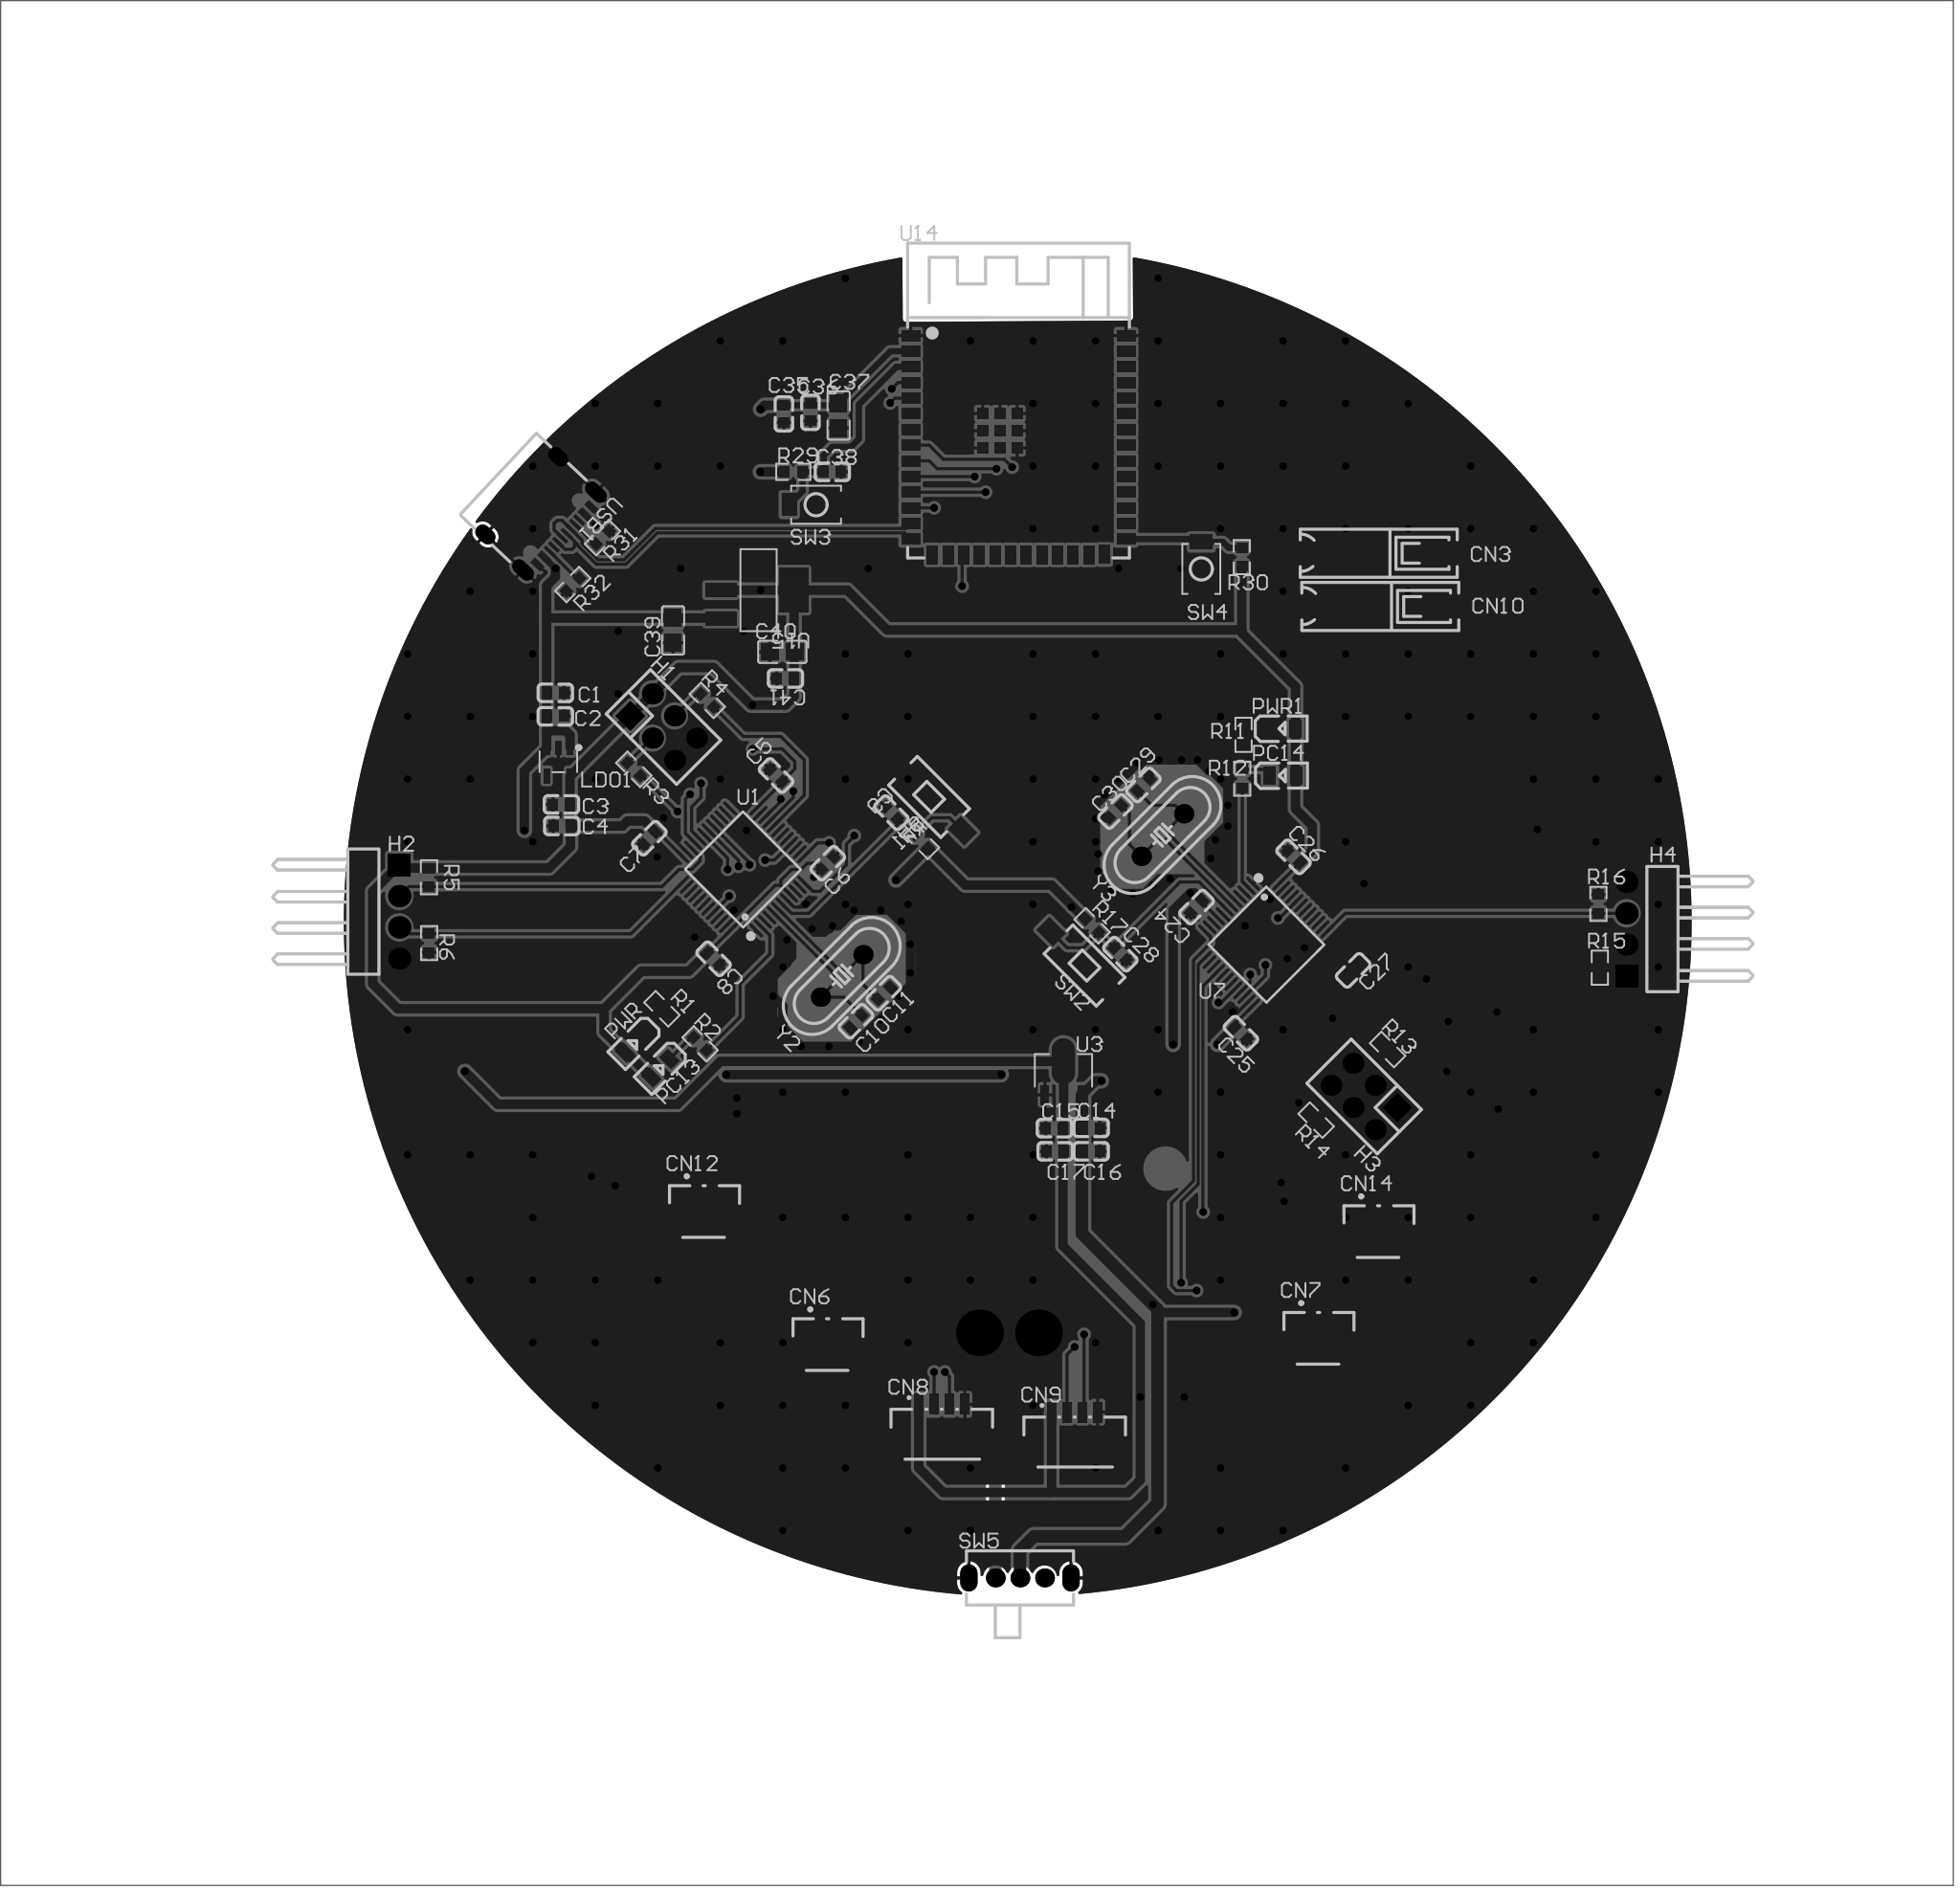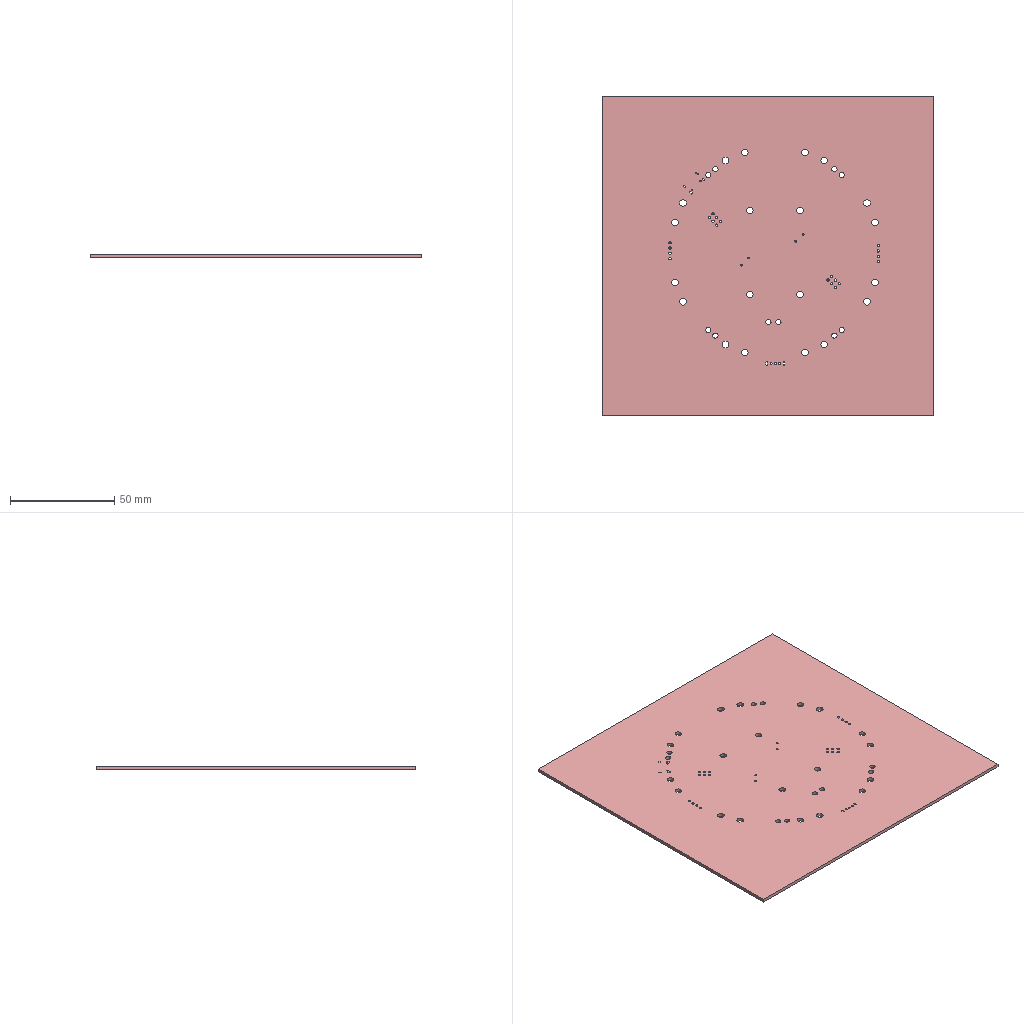Circuit board layout | Altium Designer | box 158.6 x 152.9 x 1.6 mm
Layer stack:
# Altium Designer layer stack of  (unit mm; dielectric type: 0 none, 1 core, 2 prepreg, 3 surface material)
index,name,kind,layer,copper_thickness_mm,dielectric_type,dielectric_thickness_mm,dielectric_material,dielectric_constant
0,Top Paste Mask Layer,other,,,,,,
1,Top Silkscreen Layer,other,,,,,,
2,Top Solder Mask Layer,dielectric,,,3,0.01,,3.3
3,Top Layer,copper,Top Layer,0.035,,,,
4,Dielectric1,dielectric,,,3,1.51,FR4,4.5
5,Bottom Layer,copper,Bottom Layer,0.035,,,,
6,Bottom Solder Mask Layer,dielectric,,,3,0.01,,3.3
7,Bottom Silkscreen Layer,other,,,,,,
8,Bottom Paste Mask Layer,other,,,,,,
# drill layer pairs: low layer,high layer
drill_pair,Top Layer,Bottom Layer
Part placement:
Designator,Comment,Layer,Footprint,Center-X(mm),Center-Y(mm),Rotation
C1,CAPCER0.1UF16VX5R0603,CAPCER0.1UF25VX5R0603,CAPCER0.1UF16VX7R0603,TopLayer,C0603,114.901,166.604,180
C2,1uF,TopLayer,C0603,114.901,164.699,180
C3,1uF,TopLayer,C0603,115.411,157.549,0
C4,CAPCER0.1UF16VX5R0603,CAPCER0.1UF25VX5R0603,CAPCER0.1UF16VX7R0603,TopLayer,C0603,115.442,155.796,0
C5,100nF,TopLayer,C0603,132.842,159.893,315
C6,100nF,TopLayer,C0603,137.033,152.781,225
C7,100nF,TopLayer,C0603,122.555,154.813,45
C8,100nF,TopLayer,C0603,127.762,145.034,135
C9,CAPCER0.1UF16VX5R0603,CAPCER0.1UF25VX5R0603,CAPCER0.1UF16VX7R0603,TopLayer,C0603,142.214,156.871,315
C10,18pF,TopLayer,C0603,139.319,139.954,225
C11,18pF,TopLayer,C0603,141.605,142.24,45
C14,100nF,TopLayer,C0603,158.428,131.313,180
C15,100nF,TopLayer,C0603,155.446,131.285,180
C16,10uF,TopLayer,C0603,158.428,129.408,180
C17,22uF,TopLayer,C0603,155.507,129.408,180
C18,30pF,BottomLayer,C0805,112.402,137.656,90
C19,30pF,BottomLayer,C0805,114.561,137.656,90
C24,100nF,TopLayer,C0603,167.005,149.225,45
C25,100nF,TopLayer,C0603,170.6,138.994,135
C26,100nF,TopLayer,C0603,174.879,153.289,315
C27,100nF,TopLayer,C0603,179.718,144.083,225
C28,CAPCER0.1UF16VX5R0603,CAPCER0.1UF25VX5R0603,CAPCER0.1UF16VX7R0603,TopLayer,C0603,160.805,145.414,135
C29,18pF,TopLayer,C0603,162.687,159.131,45
C30,18pF,TopLayer,C0603,160.401,156.972,225
C33,30pF,BottomLayer,C0805,193.421,154.432,90
C34,30pF,BottomLayer,C0805,189.077,158.454,270
C35,100nF,TopLayer,C0603,133.477,189.23,90
C36,100nF,TopLayer,C0603,135.636,189.357,90
C37,10uF,TopLayer,C0805,137.922,189.103,90
C38,100nF,TopLayer,C0603,137.414,184.531,180
C39,10uF,TopLayer,C0805,124.473,171.666,90
C40,22uF,TopLayer,C0805,133.35,169.926,0
C41,100nF,TopLayer,C0603,133.604,167.767,180
CN1,WAFER-GH1.25-3PLB,BottomLayer,CONN-SMD_3P-P1.25_XUNPU_WAFER-GH1.25-3PLB,126.746,117.094,180
CN2,WAFER-GH1.25-3PLB,BottomLayer,CONN-SMD_3P-P1.25_XUNPU_WAFER-GH1.25-3PLB,163.449,122.195,180
CN3,2060-451/998-404,TopLayer,CONN-SMD_L12.7-W3.9_2060-451-998-404,182.499,177.927,0
CN4,WAFER-GH1.25-2PLB,BottomLayer,CONN-TH_2P-P1.25_XUNPU_WAFER-GH1.25-2PLB,135.763,122.047,180
CN5,WAFER-GH1.25-2PLB,BottomLayer,CONN-TH_2P-P1.25_XUNPU_WAFER-GH1.25-2PLB,166.37,114.808,180
CN6,WAFER-GH1.25-2PLB,TopLayer,CONN-TH_2P-P1.25_XUNPU_WAFER-GH1.25-2PLB,137.033,114.427,0
CN7,WAFER-GH1.25-2PLB,TopLayer,CONN-TH_2P-P1.25_XUNPU_WAFER-GH1.25-2PLB,176.911,114.935,0
CN10,2060-451/998-404,TopLayer,CONN-SMD_L12.7-W3.9_2060-451-998-404,182.626,173.609,0
CN11,GH1.25-2P,BottomLayer,CONN-TH_2P-P1.25_XUNPU_WAFER-GH1.25-2PLB,119.126,122.682,180
CN12,GH1.25-2P,TopLayer,CONN-TH_2P-P1.25_XUNPU_WAFER-GH1.25-2PLB,127,125.222,0
CN13,GH1.25-2P,BottomLayer,CONN-TH_2P-P1.25_XUNPU_WAFER-GH1.25-2PLB,173.482,121.412,180
CN14,GH1.25-2P,TopLayer,CONN-TH_2P-P1.25_XUNPU_WAFER-GH1.25-2PLB,181.787,123.592,0
H1,PZ254V-12-6P,TopLayer,HDR-TH_6P-P2.54-V-M-R2-C3-S2.54,123.698,163.83,315
H2,2541WR-04P,TopLayer,HDR-TH_4P-P2.54-H-M-W10.4-N,102.235,148.844,270
H3,PZ254V-12-6P,TopLayer,HDR-TH_6P-P2.54-V-M-R2-C3-S2.54,180.617,133.857,135
H4,2541WR-04P,TopLayer,HDR-TH_4P-P2.54-H-M-W10.4-N,201.93,147.447,90
LDO1,ME6211C33M5G-N,TopLayer,SOT-23-5_L3.0-W1.7-P0.95-LS2.8-BL,115.156,161.016,180
PC13,NCD0805R1,TopLayer,LED0805-R-RD,123.444,136.144,225
PC14,NCD0805R1,TopLayer,LED0805-R-RD,174.013,159.892,0
PWR,NCD0805R1,TopLayer,LED0805-R-RD,121.306,138.167,225
PWR1,NCD0805R1,TopLayer,LED0805-R-RD,173.99,163.703,0
Q1,STD12NF06LT4,BottomLayer,TO-252-3_L6.5-W5.8-P4.58-BL,122.816,145.785,180
Q2,STD12NF06LT4,BottomLayer,TO-252-3_L6.5-W5.8-P4.58-BL,179.959,150.241,0
Q3,STD12NF06LT4,BottomLayer,TO-252-3_L6.5-W5.8-P4.58-BL,122.963,132.762,180
Q4,STD12NF06LT4,BottomLayer,TO-252-3_L6.5-W5.8-P4.58-BL,179.912,163.349,0
R1,10kΩ,TopLayer,R0603,123.571,140.97,135
R2,10kΩ,TopLayer,R0603,126.668,138.127,315
R3,10kΩ,TopLayer,R0603,121.285,160.401,135
R4,10kΩ,TopLayer,R0603,127.254,165.989,315
R5,10kΩ,TopLayer,R0603,104.648,151.638,90
R6,10kΩ,TopLayer,R0603,104.661,146.301,90
R7,10kΩ,TopLayer,R0603,144.653,154.559,315
R8,0Ω,BottomLayer,R0805,112.402,141.72,270
R9,0Ω,BottomLayer,R0805,114.561,141.72,270
R10,120Ω,BottomLayer,R0805,116.72,139.308,90
R11,10kΩ,TopLayer,R0603,170.815,163.195,270
R12,10kΩ,TopLayer,R0603,170.711,159.638,270
R13,10kΩ,TopLayer,R0603,182.522,137.667,315
R14,10kΩ,TopLayer,R0603,176.714,131.937,135
R15,10kΩ,TopLayer,R0603,199.758,144.304,270
R16,10kΩ,TopLayer,R0603,199.644,149.479,270
R17,10kΩ,TopLayer,R0603,158.519,147.7,135
R18,0Ω,BottomLayer,R0805,191.236,154.391,90
R19,0Ω,BottomLayer,R0805,189.077,154.391,90
R20,120Ω,BottomLayer,R0805,186.944,158.369,90
R21,10kΩ,BottomLayer,R0603,116.84,142.748,90
R22,10kΩ,BottomLayer,R0603,186.77,154.332,270
R27,1kΩ,BottomLayer,R0805,128.805,141.017,270
R28,1kΩ,BottomLayer,R0805,188.341,161.798,0
R29,10kΩ,TopLayer,R0603,134.239,184.531,0
R30,10kΩ,TopLayer,R0603,170.678,177.614,90
R31,5.1kΩ,TopLayer,R0603,118.745,179.197,225
R32,5.1kΩ,TopLayer,R0603,116.332,175.387,45
SW1,TS-1101-C-W,TopLayer,SW-SMD_L6.0-W3.3-LS8.0,145.161,158.242,135
SW2,TS-1101-C-W,TopLayer,SW-SMD_L6.0-W3.3-LS8.0,158.011,144.398,315
SW3,TS-1088-AR02016,TopLayer,SW-SMD_L3.9-W3.0-P4.45,136.092,181.864,180
SW4,TS-1088-AR02016,TopLayer,SW-SMD_L3.9-W3.0-P4.45,167.386,176.657,90
SW5,SK12D07VG4,TopLayer,SW-TH_SK12D07VG4,152.654,94.798,0
U1,STM32F103C8T6,TopLayer,LQFP-48_L7.0-W7.0-P0.50-LS9.0-BL,130.175,152.273,45
U2,0.1uF/100V,BottomLayer,C0805,114.815,156.548,90
U3,AMS1117-5.0,TopLayer,SOT-89-3_L4.5-W2.5-P1.50-LS4.2-BR,156.186,135.151,270
U4,TJA1050T/CM-YJLTY,BottomLayer,SOIC-8_L4.9-W3.9-P1.27-LS6.0-BL,114.18,148.833,0
U6,XT30U-F,BottomLayer,CONN-TH_XT30U-F,151.765,114.681,180
U7,STM32F103C8T6,TopLayer,LQFP-48_L7.0-W7.0-P0.50-LS9.0-BL,172.651,146.176,225
U8,TJA1050T/CM-YJLTY,BottomLayer,SOIC-8_L4.9-W3.9-P1.27-LS6.0-BL,189.458,147.279,180
U9,0.1uF/100V,BottomLayer,C0805,188.823,139.564,270
U14,2.4GHz,TopLayer,WIRELM-SMD_ESP32-S3-WROOM-1,152.527,186.69,0
U15,AMS1117-3.3,TopLayer,SOT-223-3_L6.5-W3.4-P2.30-LS7.0-BR,131.317,174.932,180
USB1,TYPE-C 16PIN 2MD(073),TopLayer,USB-C-SMD_TYPE-C-16PIN-2MD-073,113.719,181.163,226.8
Y2,8M crystal,TopLayer,HC-49S_L11.5-W4.7-P4.88,138.176,143.637,45
Y3,8M crystal,TopLayer,HC-49S_L11.5-W4.7-P4.88,164.234,155.066,225
CN8,LQ-GH1.25-4PLT,TopLayer,CONN-SMD_LQ-GH1.25-4PLT,146.304,107.188,0
CN9,LQ-GH1.25-4PLT,TopLayer,CONN-SMD_LQ-GH1.25-4PLT,157.099,106.553,0
Pad and via stacks:
# Altium Designer via and pad stacks of  (unit mm). Each distinct definition once, with the count of objects using it.
# via: kind,start_layer,end_layer,hole_mm,diameter_mm,mode(0 simple;1 top-mid-bottom;2 full stack),diameter_per_layer,count,example_net
# pad: kind,layer,hole_mm,hole_type(0 round;1 square;2 slot),plating,top_size,top_shape(1 round;2 rect;3 octagon;9 rounded rect),mid_size,bottom_size,mode,footprint,size_per_layer,count,example
pad,Top Layer,0,0,plated,0.8x0.9,2,0.8x0.9,0.8x0.9,0,C0603,,52,C1.2
pad,Top Layer,0,0,plated,1.41x1.35,2,1.41x1.35,1.41x1.35,0,C0805,,6,C37.2
pad,Top Layer,0,0,plated,3.5x1.7,2,3.5x1.7,3.5x1.7,0,CONN-SMD_L12.7-W3.9_2060-451-998-404,,2,CN3.2
pad,Top Layer,0,0,plated,6x1.7,2,6x1.7,6x1.7,0,CONN-SMD_L12.7-W3.9_2060-451-998-404,,2,CN3.1
pad,Top Layer,0,0,plated,1x2.8,2,1x2.8,1x2.8,0,CONN-TH_2P-P1.25_XUNPU_WAFER-GH1.25-2PLB,,8,CN6.4
pad,Top Layer,0,0,plated,0.6x1.7,2,0.6x1.7,0.6x1.7,0,CONN-TH_2P-P1.25_XUNPU_WAFER-GH1.25-2PLB,,8,CN6.2
pad,Top Layer,0,0,plated,0.49x1.157,2,0.49x1.157,0.49x1.157,0,SOT-23-5_L3.0-W1.7-P0.95-LS2.8-BL,,3,LDO1.1
pad,Top Layer,0,0,plated,0.49x1.175,2,0.49x1.175,0.49x1.175,0,SOT-23-5_L3.0-W1.7-P0.95-LS2.8-BL,,2,LDO1.4
pad,Top Layer,0,0,plated,1x1.399,2,1x1.399,1x1.399,0,LED0805-R-RD,,8,PC13.2
pad,Top Layer,0,0,plated,0.8065x0.864,2,0.8065x0.864,0.8065x0.864,0,R0603,,36,R1.2
pad,Top Layer,0,0,plated,1.9x1.5,2,1.9x1.5,1.9x1.5,0,SW-SMD_L6.0-W3.3-LS8.0,,4,SW1.1
pad,Top Layer,0,0,plated,1.23x1.86,2,1.23x1.86,1.23x1.86,0,SW-SMD_L3.9-W3.0-P4.45,,4,SW3.1
pad,Top Layer,0,0,plated,0.27x1.5,1,0.27x1.5,0.27x1.5,0,LQFP-48_L7.0-W7.0-P0.50-LS9.0-BL,,48,U1.1
pad,Top Layer,0,0,plated,1.5x0.27,1,1.5x0.27,1.5x0.27,0,LQFP-48_L7.0-W7.0-P0.50-LS9.0-BL,,48,U1.13
pad,Top Layer,0,0,plated,1.575x0.672,2,1.575x0.672,1.575x0.672,0,SOT-89-3_L4.5-W2.5-P1.50-LS4.2-BR,,2,U3.1
pad,Top Layer,0,0,plated,0.95x0.95,1,0.95x0.95,0.95x0.95,0,SOT-89-3_L4.5-W2.5-P1.50-LS4.2-BR,,1,U3.2
pad,Top Layer,0,0,plated,1.5x0.9,2,1.5x0.9,1.5x0.9,0,WIRELM-SMD_ESP32-S3-WROOM-1,,40,U14.1
pad,Top Layer,0,0,plated,0.9x0.9,2,0.9x0.9,0.9x0.9,0,WIRELM-SMD_ESP32-S3-WROOM-1,,9,U14.41
pad,Top Layer,0,0,plated,2.5x1.1,2,2.5x1.1,2.5x1.1,0,SOT-223-3_L6.5-W3.4-P2.30-LS7.0-BR,,3,U15.1
pad,Top Layer,0,0,plated,2.34x3.6,2,2.34x3.6,2.34x3.6,0,SOT-223-3_L6.5-W3.4-P2.30-LS7.0-BR,,1,U15.4
pad,Top Layer,0,0,plated,0.55x1.1,2,0.55x1.1,0.55x1.1,0,USB-C-SMD_TYPE-C-16PIN-2MD-073,,4,USB1.A1B12
pad,Top Layer,0,0,plated,0.3x1.1,2,0.3x1.1,0.3x1.1,0,USB-C-SMD_TYPE-C-16PIN-2MD-073,,8,USB1.B8
pad,Top Layer,0,0,plated,0.7x1.68,2,0.7x1.68,0.7x1.68,0,CONN-SMD_LQ-GH1.25-4PLT,,8,CN8.1
pad,Top Layer,0,0,plated,1x2.85,2,1x2.85,1x2.85,0,CONN-SMD_LQ-GH1.25-4PLT,,4,CN8.5
pad,Bottom Layer,0,0,plated,1.41x1.35,2,1.41x1.35,1.41x1.35,0,C0805,,12,C18.2
pad,Bottom Layer,0,0,plated,0.6x1.7,2,0.6x1.7,0.6x1.7,0,CONN-SMD_3P-P1.25_XUNPU_WAFER-GH1.25-3PLB,,6,CN1.1
pad,Bottom Layer,0,0,plated,1x2.8,2,1x2.8,1x2.8,0,CONN-SMD_3P-P1.25_XUNPU_WAFER-GH1.25-3PLB,,4,CN1.5
pad,Bottom Layer,0,0,plated,1x2.8,2,1x2.8,1x2.8,0,CONN-TH_2P-P1.25_XUNPU_WAFER-GH1.25-2PLB,,8,CN4.4
pad,Bottom Layer,0,0,plated,0.6x1.7,2,0.6x1.7,0.6x1.7,0,CONN-TH_2P-P1.25_XUNPU_WAFER-GH1.25-2PLB,,8,CN4.2
pad,Bottom Layer,0,0,plated,2.54x1.27,2,2.54x1.27,2.54x1.27,0,TO-252-3_L6.5-W5.8-P4.58-BL,,8,Q1.3
pad,Bottom Layer,0,0,plated,6.1x5.4,2,6.1x5.4,6.1x5.4,0,TO-252-3_L6.5-W5.8-P4.58-BL,,4,Q1.2
pad,Bottom Layer,0,0,plated,1.133x1.377,2,1.133x1.377,1.133x1.377,0,R0805,,16,R8.2
pad,Bottom Layer,0,0,plated,0.8065x0.864,2,0.8065x0.864,0.8065x0.864,0,R0603,,4,R21.2
pad,Bottom Layer,0,0,plated,0.588x2.045,1,0.588x2.045,0.588x2.045,0,SOIC-8_L4.9-W3.9-P1.27-LS6.0-BL,,16,U4.1
pad,Multi-Layer,1.1,0,plated,1.7x1.7,2,1.7x1.7,1.7x1.7,0,HDR-TH_6P-P2.54-V-M-R2-C3-S2.54,,2,H1.1
pad,Multi-Layer,1.1,0,plated,1.7x1.7,1,1.7x1.7,1.7x1.7,0,HDR-TH_6P-P2.54-V-M-R2-C3-S2.54,,10,H1.2
pad,Multi-Layer,1.1,0,plated,1.8x1.8,2,1.8x1.8,1.8x1.8,0,HDR-TH_4P-P2.54-H-M-W10.4-N,,2,H2.1
pad,Multi-Layer,1.1,0,plated,1.8x1.8,1,1.8x1.8,1.8x1.8,0,HDR-TH_4P-P2.54-H-M-W10.4-N,,6,H2.2
pad,Multi-Layer,0.9144,0,plated,1.524x1.524,1,1.524x1.524,1.524x1.524,0,SW-TH_SK12D07VG4,,3,SW5.1
pad,Multi-Layer,0.8,2,plated,1.4x2.2,1,1.4x2.2,1.4x2.2,0,SW-TH_SK12D07VG4,,2,SW5.4
pad,Multi-Layer,2.54,0,plated,3.8x3.8,1,3.8x3.8,3.8x3.8,0,CONN-TH_XT30U-F,,2,U6.1
pad,Multi-Layer,0.6,2,plated,1.1x2,1,1.1x2,1.1x2,0,USB-C-SMD_TYPE-C-16PIN-2MD-073,,2,USB1.13
pad,Multi-Layer,0.6,2,plated,1.2x1.8,1,1.2x1.8,1.2x1.8,0,USB-C-SMD_TYPE-C-16PIN-2MD-073,,2,USB1.13
pad,Multi-Layer,0.9,0,plated,1.56x1.56,1,1.56x1.56,1.56x1.56,0,HC-49S_L11.5-W4.7-P4.88,,4,Y2.2
via,Top Layer,Bottom Layer,0.3048,0.6096,0,,293,BOOT0
Copper pours:
name,layer,net,type(0 solid;1 hatched;2 none)
Top Layer-GND,Top Layer,GND,0
Bottom Layer-GND,Bottom Layer,GND,0
Design rules, without the lines most boards share:
# Altium Designer design rules of  (exported by Altium Designer, unit mm)
# columns: name | kind | enabled | priority | scope1 | scope2 | descriptor | typed fields (field=value)
copperThickness2oz | 0 | disabled | 1 | All | All | Clearance Constraint (Gap=6mil) (Disabled)(All),(All) | gap=0.1524
Plane_innerPlane | 0 | disabled | 2 | All | All | Clearance Constraint (Gap=6mil) (Disabled)(All),(All) | gap=0.1524
Copper_copperRegion | 0 | disabled | 3 | All | All | Clearance Constraint (Gap=6mil) (Disabled)(All),(All) | gap=0.1524
copperThickness1oz | 0 | enabled | 4 | All | All | Clearance Constraint (Gap=6mil) (All),(All) | gap=0.1524
otherClearance | 52 | enabled | 1 | All | All | Hole To Hole Clearance (Gap=11.8mil) (All),(All) | gap=0.2997
5V | 2 | enabled | 2 | (InNet('+5V')) | All | Width Constraint (Min=15mil) (Max=30mil) (Preferred=15mil) ((InNet('+5V'))) |
OUTPUT | 2 | enabled | 3 | (InNet('OUTPUT')) | All | Width Constraint (Min=30mil) (Max=100mil) (Preferred=40mil) ((InNet('OUTPUT'))) |
POWER | 2 | enabled | 4 | (InNet('POWER')) | All | Width Constraint (Min=40mil) (Max=100mil) (Preferred=50mil) ((InNet('POWER'))) |
copperThickness1oz_2 | 2 | enabled | 5 | All | All | Width Constraint (Min=10mil) (Max=30mil) (Preferred=10mil) (All) |
viaSize | 11 | enabled | 1 | All | All | Routing Via (MinHoleWidth=11.8mil) (MaxHoleWidth=248mil) (PreferredHoleWidth=12mil) (MinWidth=19.7mil) (MaxWidth=393.7mil) (PreferedWidth=24mil) (All) | via_min_hole=0.2997 via_max_hole=6.299 via_preferred_diameter=0.6096 via_preferred_hole=0.3048